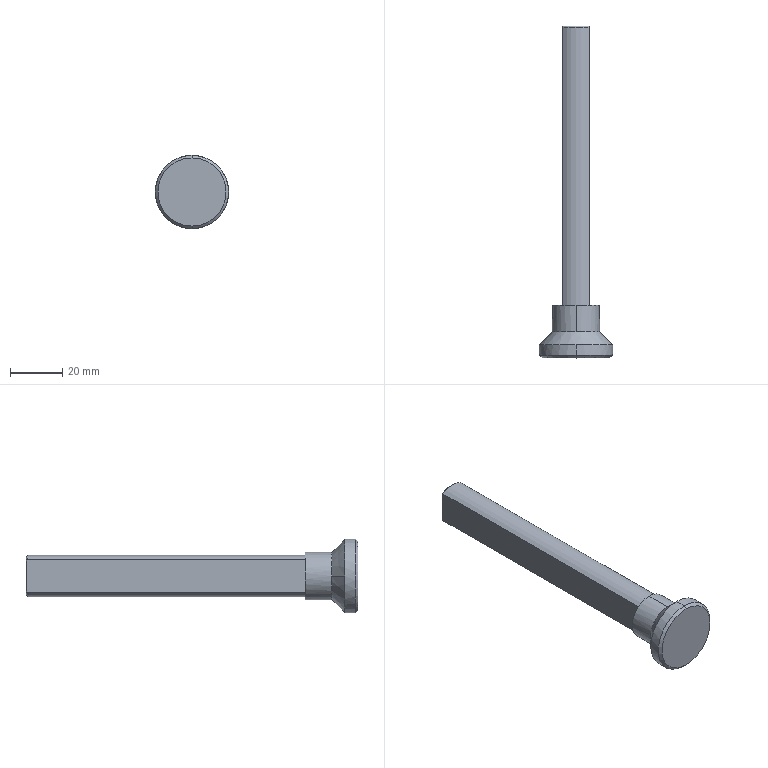Part | STEP file | PN_0017 Snap-ring stop plate | 1 solid | 19 faces | box 28 x 126.5 x 28 mm | volume 23542 mm3 | cylinder 7 | cone 7 | plane 5 | commonest cylinder face diameters 16 x3 18 x2 28 x2
STEP:
#1=CARTESIAN_POINT('',(0.,0.,0.));
#2=DIRECTION('',(0.,0.,1.));
#3=DIRECTION('',(1.,0.,0.));
#4=AXIS2_PLACEMENT_3D('',#1,#2,#3);
#5=CARTESIAN_POINT('',(-5.,106.,-6.245));
#6=VERTEX_POINT('',#5);
#7=CARTESIAN_POINT('',(0.,106.,-8.));
#8=VERTEX_POINT('',#7);
#9=CARTESIAN_POINT('',(0.,106.,0.));
#10=DIRECTION('',(0.,-1.,0.));
#11=DIRECTION('',(0.,0.,-1.));
#12=AXIS2_PLACEMENT_3D('',#9,#10,#11);
#13=CIRCLE('',#12,8.);
#14=CARTESIAN_POINT('',(0.,106.5,0.));
#15=DIRECTION('',(0.,-1.,0.));
#16=DIRECTION('',(0.,0.,-1.));
#17=AXIS2_PLACEMENT_3D('',#14,#15,#16);
#18=CYLINDRICAL_SURFACE('',#17,8.);
#19=CARTESIAN_POINT('',(0.,0.5));
#20=DIRECTION('',(1.,0.));
#21=VECTOR('',#20,1.);
#22=LINE('',#19,#21);
#23=(GEOMETRIC_REPRESENTATION_CONTEXT(2)PARAMETRIC_REPRESENTATION_CONTEXT()REPRESENTATION_CONTEXT('',''));
#24=DEFINITIONAL_REPRESENTATION('',(#22),#23);
#25=PCURVE('',#18,#24);
#26=CARTESIAN_POINT('',(0.,106.,0.));
#27=DIRECTION('',(0.,-1.,0.));
#28=DIRECTION('',(0.,0.,-1.));
#29=AXIS2_PLACEMENT_3D('',#26,#27,#28);
#30=CONICAL_SURFACE('',#29,8.,0.7854);
#31=CARTESIAN_POINT('',(0.,0.));
#32=DIRECTION('',(1.,0.));
#33=VECTOR('',#32,1.);
#34=LINE('',#31,#33);
#35=(GEOMETRIC_REPRESENTATION_CONTEXT(2)PARAMETRIC_REPRESENTATION_CONTEXT()REPRESENTATION_CONTEXT('',''));
#36=DEFINITIONAL_REPRESENTATION('',(#34),#35);
#37=PCURVE('',#30,#36);
#38=SURFACE_CURVE('',#13,(#25,#37),.PCURVE_S1.);
#39=EDGE_CURVE('',#6,#8,#38,.T.);
#40=ORIENTED_EDGE('',*,*,#39,.T.);
#41=CARTESIAN_POINT('',(0.,0.,-8.));
#42=VERTEX_POINT('',#41);
#43=CARTESIAN_POINT('',(0.,106.5,-8.));
#44=DIRECTION('',(0.,-1.,0.));
#45=VECTOR('',#44,1.);
#46=LINE('',#43,#45);
#47=CARTESIAN_POINT('',(6.283,0.));
#48=DIRECTION('',(0.,1.));
#49=VECTOR('',#48,1.);
#50=LINE('',#47,#49);
#51=(GEOMETRIC_REPRESENTATION_CONTEXT(2)PARAMETRIC_REPRESENTATION_CONTEXT()REPRESENTATION_CONTEXT('',''));
#52=DEFINITIONAL_REPRESENTATION('',(#50),#51);
#53=PCURVE('',#18,#52);
#54=CARTESIAN_POINT('',(0.,106.5,0.));
#55=DIRECTION('',(0.,-1.,0.));
#56=DIRECTION('',(0.,0.,-1.));
#57=AXIS2_PLACEMENT_3D('',#54,#55,#56);
#58=CYLINDRICAL_SURFACE('',#57,8.);
#59=CARTESIAN_POINT('',(0.,0.));
#60=DIRECTION('',(0.,1.));
#61=VECTOR('',#60,1.);
#62=LINE('',#59,#61);
#63=(GEOMETRIC_REPRESENTATION_CONTEXT(2)PARAMETRIC_REPRESENTATION_CONTEXT()REPRESENTATION_CONTEXT('',''));
#64=DEFINITIONAL_REPRESENTATION('',(#62),#63);
#65=PCURVE('',#58,#64);
#66=SURFACE_CURVE('',#46,(#53,#65),.PCURVE_S1.);
#67=EDGE_CURVE('',#8,#42,#66,.T.);
#68=ORIENTED_EDGE('',*,*,#67,.T.);
#69=CARTESIAN_POINT('',(-5.,0.,-6.245));
#70=VERTEX_POINT('',#69);
#71=CARTESIAN_POINT('',(0.,0.,0.));
#72=DIRECTION('',(0.,1.,0.));
#73=DIRECTION('',(0.,0.,-1.));
#74=AXIS2_PLACEMENT_3D('',#71,#72,#73);
#75=CIRCLE('',#74,8.);
#76=CARTESIAN_POINT('',(6.283,106.5));
#77=DIRECTION('',(-1.,0.));
#78=VECTOR('',#77,1.);
#79=LINE('',#76,#78);
#80=(GEOMETRIC_REPRESENTATION_CONTEXT(2)PARAMETRIC_REPRESENTATION_CONTEXT()REPRESENTATION_CONTEXT('',''));
#81=DEFINITIONAL_REPRESENTATION('',(#79),#80);
#82=PCURVE('',#18,#81);
#83=CARTESIAN_POINT('',(0.,0.,0.));
#84=DIRECTION('',(0.,-1.,0.));
#85=DIRECTION('',(0.,0.,-1.));
#86=AXIS2_PLACEMENT_3D('',#83,#84,#85);
#87=PLANE('',#86);
#88=CARTESIAN_POINT('',(8.,0.));
#89=CARTESIAN_POINT('',(8.,-13.856));
#90=CARTESIAN_POINT('',(-4.,-6.928));
#91=CARTESIAN_POINT('',(-16.,0.));
#92=CARTESIAN_POINT('',(-4.,6.928));
#93=CARTESIAN_POINT('',(8.,13.856));
#94=CARTESIAN_POINT('',(8.,0.));
#95=(BOUNDED_CURVE()B_SPLINE_CURVE(2,(#88,#89,#90,#91,#92,#93,#94),.UNSPECIFIED.,.T.,.F.)B_SPLINE_CURVE_WITH_KNOTS((1,2,2,2,2,1),(-2.094,0.,2.094,4.189,6.283,8.378),.UNSPECIFIED.)CURVE()GEOMETRIC_REPRESENTATION_ITEM()RATIONAL_B_SPLINE_CURVE((1.,0.5,1.,0.5,1.,0.5,1.))REPRESENTATION_ITEM(''));
#96=(GEOMETRIC_REPRESENTATION_CONTEXT(2)PARAMETRIC_REPRESENTATION_CONTEXT()REPRESENTATION_CONTEXT('',''));
#97=DEFINITIONAL_REPRESENTATION('',(#95),#96);
#98=PCURVE('',#87,#97);
#99=SURFACE_CURVE('',#75,(#82,#98),.PCURVE_S1.);
#100=EDGE_CURVE('',#42,#70,#99,.T.);
#101=ORIENTED_EDGE('',*,*,#100,.T.);
#102=CARTESIAN_POINT('',(-5.,-39.994,-6.245));
#103=DIRECTION('',(0.,-1.,0.));
#104=VECTOR('',#103,1.);
#105=LINE('',#102,#104);
#106=CARTESIAN_POINT('',(5.608,146.494));
#107=DIRECTION('',(0.,1.));
#108=VECTOR('',#107,1.);
#109=LINE('',#106,#108);
#110=(GEOMETRIC_REPRESENTATION_CONTEXT(2)PARAMETRIC_REPRESENTATION_CONTEXT()REPRESENTATION_CONTEXT('',''));
#111=DEFINITIONAL_REPRESENTATION('',(#109),#110);
#112=PCURVE('',#18,#111);
#113=CARTESIAN_POINT('',(-5.,-39.994,-10.));
#114=DIRECTION('',(-1.,0.,0.));
#115=DIRECTION('',(0.,0.,1.));
#116=AXIS2_PLACEMENT_3D('',#113,#114,#115);
#117=PLANE('',#116);
#118=CARTESIAN_POINT('',(3.755,0.));
#119=DIRECTION('',(0.,-1.));
#120=VECTOR('',#119,1.);
#121=LINE('',#118,#120);
#122=(GEOMETRIC_REPRESENTATION_CONTEXT(2)PARAMETRIC_REPRESENTATION_CONTEXT()REPRESENTATION_CONTEXT('',''));
#123=DEFINITIONAL_REPRESENTATION('',(#121),#122);
#124=PCURVE('',#117,#123);
#125=SURFACE_CURVE('',#105,(#112,#124),.PCURVE_S1.);
#126=EDGE_CURVE('',#6,#70,#125,.T.);
#127=ORIENTED_EDGE('',*,*,#126,.F.);
#128=EDGE_LOOP('',(#40,#68,#101,#127));
#129=FACE_BOUND('',#128,.T.);
#130=ADVANCED_FACE('',(#129),#18,.T.);
#131=CARTESIAN_POINT('',(0.,106.5,-7.5));
#132=VERTEX_POINT('',#131);
#133=CARTESIAN_POINT('',(-5.,106.5,-5.59));
#134=VERTEX_POINT('',#133);
#135=CARTESIAN_POINT('',(0.,106.5,0.));
#136=DIRECTION('',(0.,1.,0.));
#137=DIRECTION('',(0.,0.,-1.));
#138=AXIS2_PLACEMENT_3D('',#135,#136,#137);
#139=CIRCLE('',#138,7.5);
#140=CARTESIAN_POINT('',(6.283,-0.5));
#141=DIRECTION('',(-1.,0.));
#142=VECTOR('',#141,1.);
#143=LINE('',#140,#142);
#144=(GEOMETRIC_REPRESENTATION_CONTEXT(2)PARAMETRIC_REPRESENTATION_CONTEXT()REPRESENTATION_CONTEXT('',''));
#145=DEFINITIONAL_REPRESENTATION('',(#143),#144);
#146=PCURVE('',#30,#145);
#147=CARTESIAN_POINT('',(0.,106.5,0.));
#148=DIRECTION('',(0.,1.,0.));
#149=DIRECTION('',(0.,0.,1.));
#150=AXIS2_PLACEMENT_3D('',#147,#148,#149);
#151=PLANE('',#150);
#152=CARTESIAN_POINT('',(0.,0.));
#153=DIRECTION('',(-1.,0.));
#154=AXIS2_PLACEMENT_2D('',#152,#153);
#155=CIRCLE('',#154,7.5);
#156=(GEOMETRIC_REPRESENTATION_CONTEXT(2)PARAMETRIC_REPRESENTATION_CONTEXT()REPRESENTATION_CONTEXT('',''));
#157=DEFINITIONAL_REPRESENTATION('',(#155),#156);
#158=PCURVE('',#151,#157);
#159=SURFACE_CURVE('',#139,(#146,#158),.PCURVE_S1.);
#160=EDGE_CURVE('',#132,#134,#159,.T.);
#161=ORIENTED_EDGE('',*,*,#160,.F.);
#162=CARTESIAN_POINT('',(0.,106.,-8.));
#163=DIRECTION('',(0.,-0.7071,-0.7071));
#164=VECTOR('',#163,1.);
#165=LINE('',#162,#164);
#166=CARTESIAN_POINT('',(6.283,0.));
#167=DIRECTION('',(0.,1.));
#168=VECTOR('',#167,1.);
#169=LINE('',#166,#168);
#170=(GEOMETRIC_REPRESENTATION_CONTEXT(2)PARAMETRIC_REPRESENTATION_CONTEXT()REPRESENTATION_CONTEXT('',''));
#171=DEFINITIONAL_REPRESENTATION('',(#169),#170);
#172=PCURVE('',#30,#171);
#173=CARTESIAN_POINT('',(0.,106.,0.));
#174=DIRECTION('',(0.,-1.,0.));
#175=DIRECTION('',(0.,0.,-1.));
#176=AXIS2_PLACEMENT_3D('',#173,#174,#175);
#177=CONICAL_SURFACE('',#176,8.,0.7854);
#178=CARTESIAN_POINT('',(0.,0.));
#179=DIRECTION('',(0.,1.));
#180=VECTOR('',#179,1.);
#181=LINE('',#178,#180);
#182=(GEOMETRIC_REPRESENTATION_CONTEXT(2)PARAMETRIC_REPRESENTATION_CONTEXT()REPRESENTATION_CONTEXT('',''));
#183=DEFINITIONAL_REPRESENTATION('',(#181),#182);
#184=PCURVE('',#177,#183);
#185=SURFACE_CURVE('',#165,(#172,#184),.PCURVE_S1.);
#186=EDGE_CURVE('',#132,#8,#185,.T.);
#187=ORIENTED_EDGE('',*,*,#186,.T.);
#188=ORIENTED_EDGE('',*,*,#39,.F.);
#189=CARTESIAN_POINT('',(-5.,106.,-6.245));
#190=CARTESIAN_POINT('',(-5.,106.169,-6.029));
#191=CARTESIAN_POINT('',(-5.,106.336,-5.81));
#192=CARTESIAN_POINT('',(-5.,106.5,-5.59));
#193=B_SPLINE_CURVE_WITH_KNOTS('',3,(#189,#190,#191,#192),.UNSPECIFIED.,.F.,.F.,(4,4),(0.,0.0008239),.PIECEWISE_BEZIER_KNOTS.);
#194=CARTESIAN_POINT('',(5.608,0.));
#195=CARTESIAN_POINT('',(5.607,-0.007681));
#196=CARTESIAN_POINT('',(5.606,-0.02304));
#197=CARTESIAN_POINT('',(5.603,-0.04604));
#198=CARTESIAN_POINT('',(5.601,-0.06902));
#199=CARTESIAN_POINT('',(5.599,-0.09197));
#200=CARTESIAN_POINT('',(5.596,-0.1149));
#201=CARTESIAN_POINT('',(5.594,-0.1378));
#202=CARTESIAN_POINT('',(5.592,-0.1607));
#203=CARTESIAN_POINT('',(5.589,-0.1835));
#204=CARTESIAN_POINT('',(5.587,-0.2063));
#205=CARTESIAN_POINT('',(5.584,-0.2291));
#206=CARTESIAN_POINT('',(5.582,-0.2518));
#207=CARTESIAN_POINT('',(5.579,-0.2745));
#208=CARTESIAN_POINT('',(5.577,-0.2972));
#209=CARTESIAN_POINT('',(5.574,-0.3199));
#210=CARTESIAN_POINT('',(5.572,-0.3425));
#211=CARTESIAN_POINT('',(5.569,-0.3651));
#212=CARTESIAN_POINT('',(5.567,-0.3877));
#213=CARTESIAN_POINT('',(5.564,-0.4102));
#214=CARTESIAN_POINT('',(5.561,-0.4327));
#215=CARTESIAN_POINT('',(5.559,-0.4552));
#216=CARTESIAN_POINT('',(5.556,-0.4776));
#217=CARTESIAN_POINT('',(5.554,-0.4925));
#218=CARTESIAN_POINT('',(5.553,-0.5));
#219=B_SPLINE_CURVE_WITH_KNOTS('',3,(#194,#195,#196,#197,#198,#199,#200,#201,#202,#203,#204,#205,#206,#207,#208,#209,#210,#211,#212,#213,#214,#215,#216,#217,#218),.UNSPECIFIED.,.F.,.F.,(4,1,1,1,1,1,1,1,1,1,1,1,1,1,1,1,1,1,1,1,1,1,4),(0.,0.00003745,0.0000749,0.0001123,0.0001498,0.0001872,0.0002247,0.0002621,0.0002996,0.000337,0.0003745,0.0004119,0.0004494,0.0004868,0.0005243,0.0005617,0.0005992,0.0006366,0.0006741,0.0007115,0.000749,0.0007864,0.0008239),.QUASI_UNIFORM_KNOTS.);
#220=(GEOMETRIC_REPRESENTATION_CONTEXT(2)PARAMETRIC_REPRESENTATION_CONTEXT()REPRESENTATION_CONTEXT('',''));
#221=DEFINITIONAL_REPRESENTATION('',(#219),#220);
#222=PCURVE('',#30,#221);
#223=CARTESIAN_POINT('',(3.755,145.994));
#224=CARTESIAN_POINT('',(3.971,146.163));
#225=CARTESIAN_POINT('',(4.19,146.33));
#226=CARTESIAN_POINT('',(4.41,146.494));
#227=B_SPLINE_CURVE_WITH_KNOTS('',3,(#223,#224,#225,#226),.UNSPECIFIED.,.F.,.F.,(4,4),(0.,0.0008239),.PIECEWISE_BEZIER_KNOTS.);
#228=(GEOMETRIC_REPRESENTATION_CONTEXT(2)PARAMETRIC_REPRESENTATION_CONTEXT()REPRESENTATION_CONTEXT('',''));
#229=DEFINITIONAL_REPRESENTATION('',(#227),#228);
#230=PCURVE('',#117,#229);
#231=SURFACE_CURVE('',#193,(#222,#230),.PCURVE_S1.);
#232=EDGE_CURVE('',#6,#134,#231,.T.);
#233=ORIENTED_EDGE('',*,*,#232,.T.);
#234=EDGE_LOOP('',(#161,#187,#188,#233));
#235=FACE_BOUND('',#234,.T.);
#236=ADVANCED_FACE('',(#235),#30,.T.);
#237=CARTESIAN_POINT('',(9.,-10.,0.));
#238=VERTEX_POINT('',#237);
#239=CARTESIAN_POINT('',(0.,-10.,-9.));
#240=VERTEX_POINT('',#239);
#241=CARTESIAN_POINT('',(0.,-10.,0.));
#242=DIRECTION('',(0.,1.,0.));
#243=DIRECTION('',(0.,0.,1.));
#244=AXIS2_PLACEMENT_3D('',#241,#242,#243);
#245=CIRCLE('',#244,9.);
#246=CARTESIAN_POINT('',(0.,-15.,0.));
#247=DIRECTION('',(0.,1.,0.));
#248=DIRECTION('',(0.,0.,1.));
#249=AXIS2_PLACEMENT_3D('',#246,#247,#248);
#250=CYLINDRICAL_SURFACE('',#249,9.);
#251=CARTESIAN_POINT('',(0.,5.));
#252=DIRECTION('',(1.,0.));
#253=VECTOR('',#252,1.);
#254=LINE('',#251,#253);
#255=(GEOMETRIC_REPRESENTATION_CONTEXT(2)PARAMETRIC_REPRESENTATION_CONTEXT()REPRESENTATION_CONTEXT('',''));
#256=DEFINITIONAL_REPRESENTATION('',(#254),#255);
#257=PCURVE('',#250,#256);
#258=CARTESIAN_POINT('',(0.,-15.,0.));
#259=DIRECTION('',(0.,-1.,0.));
#260=DIRECTION('',(1.,0.,0.));
#261=AXIS2_PLACEMENT_3D('',#258,#259,#260);
#262=CONICAL_SURFACE('',#261,14.,0.7854);
#263=CARTESIAN_POINT('',(7.854,-5.));
#264=DIRECTION('',(-1.,0.));
#265=VECTOR('',#264,1.);
#266=LINE('',#263,#265);
#267=(GEOMETRIC_REPRESENTATION_CONTEXT(2)PARAMETRIC_REPRESENTATION_CONTEXT()REPRESENTATION_CONTEXT('',''));
#268=DEFINITIONAL_REPRESENTATION('',(#266),#267);
#269=PCURVE('',#262,#268);
#270=SURFACE_CURVE('',#245,(#257,#269),.PCURVE_S1.);
#271=EDGE_CURVE('',#238,#240,#270,.T.);
#272=ORIENTED_EDGE('',*,*,#271,.T.);
#273=CARTESIAN_POINT('',(0.,0.,-9.));
#274=VERTEX_POINT('',#273);
#275=CARTESIAN_POINT('',(0.,-15.,-9.));
#276=DIRECTION('',(0.,1.,0.));
#277=VECTOR('',#276,1.);
#278=LINE('',#275,#277);
#279=CARTESIAN_POINT('',(3.142,0.));
#280=DIRECTION('',(0.,1.));
#281=VECTOR('',#280,1.);
#282=LINE('',#279,#281);
#283=(GEOMETRIC_REPRESENTATION_CONTEXT(2)PARAMETRIC_REPRESENTATION_CONTEXT()REPRESENTATION_CONTEXT('',''));
#284=DEFINITIONAL_REPRESENTATION('',(#282),#283);
#285=PCURVE('',#250,#284);
#286=CARTESIAN_POINT('',(0.,-15.,0.));
#287=DIRECTION('',(0.,1.,0.));
#288=DIRECTION('',(0.,0.,1.));
#289=AXIS2_PLACEMENT_3D('',#286,#287,#288);
#290=CYLINDRICAL_SURFACE('',#289,9.);
#291=CARTESIAN_POINT('',(3.142,0.));
#292=DIRECTION('',(0.,1.));
#293=VECTOR('',#292,1.);
#294=LINE('',#291,#293);
#295=(GEOMETRIC_REPRESENTATION_CONTEXT(2)PARAMETRIC_REPRESENTATION_CONTEXT()REPRESENTATION_CONTEXT('',''));
#296=DEFINITIONAL_REPRESENTATION('',(#294),#295);
#297=PCURVE('',#290,#296);
#298=SURFACE_CURVE('',#278,(#285,#297),.PCURVE_S1.);
#299=EDGE_CURVE('',#240,#274,#298,.T.);
#300=ORIENTED_EDGE('',*,*,#299,.T.);
#301=CARTESIAN_POINT('',(0.,0.,9.));
#302=VERTEX_POINT('',#301);
#303=CARTESIAN_POINT('',(0.,0.,0.));
#304=DIRECTION('',(0.,-1.,0.));
#305=DIRECTION('',(0.,0.,1.));
#306=AXIS2_PLACEMENT_3D('',#303,#304,#305);
#307=CIRCLE('',#306,9.);
#308=CARTESIAN_POINT('',(6.283,15.));
#309=DIRECTION('',(-1.,0.));
#310=VECTOR('',#309,1.);
#311=LINE('',#308,#310);
#312=(GEOMETRIC_REPRESENTATION_CONTEXT(2)PARAMETRIC_REPRESENTATION_CONTEXT()REPRESENTATION_CONTEXT('',''));
#313=DEFINITIONAL_REPRESENTATION('',(#311),#312);
#314=PCURVE('',#250,#313);
#315=CARTESIAN_POINT('',(0.,0.));
#316=DIRECTION('',(-1.,0.));
#317=AXIS2_PLACEMENT_2D('',#315,#316);
#318=CIRCLE('',#317,9.);
#319=(GEOMETRIC_REPRESENTATION_CONTEXT(2)PARAMETRIC_REPRESENTATION_CONTEXT()REPRESENTATION_CONTEXT('',''));
#320=DEFINITIONAL_REPRESENTATION('',(#318),#319);
#321=PCURVE('',#87,#320);
#322=SURFACE_CURVE('',#307,(#314,#321),.PCURVE_S1.);
#323=EDGE_CURVE('',#274,#302,#322,.T.);
#324=ORIENTED_EDGE('',*,*,#323,.T.);
#325=CARTESIAN_POINT('',(0.,-10.,9.));
#326=VERTEX_POINT('',#325);
#327=CARTESIAN_POINT('',(0.,-15.,9.));
#328=DIRECTION('',(0.,1.,0.));
#329=VECTOR('',#328,1.);
#330=LINE('',#327,#329);
#331=CARTESIAN_POINT('',(0.,0.));
#332=DIRECTION('',(0.,1.));
#333=VECTOR('',#332,1.);
#334=LINE('',#331,#333);
#335=(GEOMETRIC_REPRESENTATION_CONTEXT(2)PARAMETRIC_REPRESENTATION_CONTEXT()REPRESENTATION_CONTEXT('',''));
#336=DEFINITIONAL_REPRESENTATION('',(#334),#335);
#337=PCURVE('',#250,#336);
#338=CARTESIAN_POINT('',(6.283,0.));
#339=DIRECTION('',(0.,1.));
#340=VECTOR('',#339,1.);
#341=LINE('',#338,#340);
#342=(GEOMETRIC_REPRESENTATION_CONTEXT(2)PARAMETRIC_REPRESENTATION_CONTEXT()REPRESENTATION_CONTEXT('',''));
#343=DEFINITIONAL_REPRESENTATION('',(#341),#342);
#344=PCURVE('',#290,#343);
#345=SURFACE_CURVE('',#330,(#337,#344),.PCURVE_S1.);
#346=EDGE_CURVE('',#326,#302,#345,.T.);
#347=ORIENTED_EDGE('',*,*,#346,.F.);
#348=CARTESIAN_POINT('',(0.,-10.,0.));
#349=DIRECTION('',(0.,1.,0.));
#350=DIRECTION('',(0.,0.,1.));
#351=AXIS2_PLACEMENT_3D('',#348,#349,#350);
#352=CIRCLE('',#351,9.);
#353=CARTESIAN_POINT('',(0.,5.));
#354=DIRECTION('',(1.,0.));
#355=VECTOR('',#354,1.);
#356=LINE('',#353,#355);
#357=(GEOMETRIC_REPRESENTATION_CONTEXT(2)PARAMETRIC_REPRESENTATION_CONTEXT()REPRESENTATION_CONTEXT('',''));
#358=DEFINITIONAL_REPRESENTATION('',(#356),#357);
#359=PCURVE('',#250,#358);
#360=CARTESIAN_POINT('',(0.,-15.,0.));
#361=DIRECTION('',(0.,-1.,0.));
#362=DIRECTION('',(1.,0.,0.));
#363=AXIS2_PLACEMENT_3D('',#360,#361,#362);
#364=CONICAL_SURFACE('',#363,14.,0.7854);
#365=CARTESIAN_POINT('',(1.571,-5.));
#366=DIRECTION('',(-1.,0.));
#367=VECTOR('',#366,1.);
#368=LINE('',#365,#367);
#369=(GEOMETRIC_REPRESENTATION_CONTEXT(2)PARAMETRIC_REPRESENTATION_CONTEXT()REPRESENTATION_CONTEXT('',''));
#370=DEFINITIONAL_REPRESENTATION('',(#368),#369);
#371=PCURVE('',#364,#370);
#372=SURFACE_CURVE('',#352,(#359,#371),.PCURVE_S1.);
#373=EDGE_CURVE('',#326,#238,#372,.T.);
#374=ORIENTED_EDGE('',*,*,#373,.T.);
#375=EDGE_LOOP('',(#272,#300,#324,#347,#374));
#376=FACE_BOUND('',#375,.T.);
#377=ADVANCED_FACE('',(#376),#250,.T.);
#378=CARTESIAN_POINT('',(-9.,-10.,0.));
#379=VERTEX_POINT('',#378);
#380=CARTESIAN_POINT('',(0.,-10.,0.));
#381=DIRECTION('',(0.,1.,0.));
#382=DIRECTION('',(0.,0.,1.));
#383=AXIS2_PLACEMENT_3D('',#380,#381,#382);
#384=CIRCLE('',#383,9.);
#385=CARTESIAN_POINT('',(7.854,-5.));
#386=DIRECTION('',(-1.,0.));
#387=VECTOR('',#386,1.);
#388=LINE('',#385,#387);
#389=(GEOMETRIC_REPRESENTATION_CONTEXT(2)PARAMETRIC_REPRESENTATION_CONTEXT()REPRESENTATION_CONTEXT('',''));
#390=DEFINITIONAL_REPRESENTATION('',(#388),#389);
#391=PCURVE('',#364,#390);
#392=CARTESIAN_POINT('',(0.,5.));
#393=DIRECTION('',(1.,0.));
#394=VECTOR('',#393,1.);
#395=LINE('',#392,#394);
#396=(GEOMETRIC_REPRESENTATION_CONTEXT(2)PARAMETRIC_REPRESENTATION_CONTEXT()REPRESENTATION_CONTEXT('',''));
#397=DEFINITIONAL_REPRESENTATION('',(#395),#396);
#398=PCURVE('',#290,#397);
#399=SURFACE_CURVE('',#384,(#391,#398),.PCURVE_S1.);
#400=EDGE_CURVE('',#379,#326,#399,.T.);
#401=ORIENTED_EDGE('',*,*,#400,.F.);
#402=CARTESIAN_POINT('',(-14.,-15.,0.));
#403=VERTEX_POINT('',#402);
#404=CARTESIAN_POINT('',(-14.,-15.,0.));
#405=DIRECTION('',(-0.7071,-0.7071,0.));
#406=VECTOR('',#405,1.);
#407=LINE('',#404,#406);
#408=CARTESIAN_POINT('',(3.142,0.));
#409=DIRECTION('',(0.,1.));
#410=VECTOR('',#409,1.);
#411=LINE('',#408,#410);
#412=(GEOMETRIC_REPRESENTATION_CONTEXT(2)PARAMETRIC_REPRESENTATION_CONTEXT()REPRESENTATION_CONTEXT('',''));
#413=DEFINITIONAL_REPRESENTATION('',(#411),#412);
#414=PCURVE('',#364,#413);
#415=CARTESIAN_POINT('',(3.142,0.));
#416=DIRECTION('',(0.,1.));
#417=VECTOR('',#416,1.);
#418=LINE('',#415,#417);
#419=(GEOMETRIC_REPRESENTATION_CONTEXT(2)PARAMETRIC_REPRESENTATION_CONTEXT()REPRESENTATION_CONTEXT('',''));
#420=DEFINITIONAL_REPRESENTATION('',(#418),#419);
#421=PCURVE('',#262,#420);
#422=SURFACE_CURVE('',#407,(#414,#421),.PCURVE_S1.);
#423=EDGE_CURVE('',#379,#403,#422,.T.);
#424=ORIENTED_EDGE('',*,*,#423,.T.);
#425=CARTESIAN_POINT('',(0.,-15.,14.));
#426=VERTEX_POINT('',#425);
#427=CARTESIAN_POINT('',(0.,-15.,0.));
#428=DIRECTION('',(0.,1.,0.));
#429=DIRECTION('',(0.,0.,-1.));
#430=AXIS2_PLACEMENT_3D('',#427,#428,#429);
#431=CIRCLE('',#430,14.);
#432=CARTESIAN_POINT('',(4.712,0.));
#433=DIRECTION('',(-1.,0.));
#434=VECTOR('',#433,1.);
#435=LINE('',#432,#434);
#436=(GEOMETRIC_REPRESENTATION_CONTEXT(2)PARAMETRIC_REPRESENTATION_CONTEXT()REPRESENTATION_CONTEXT('',''));
#437=DEFINITIONAL_REPRESENTATION('',(#435),#436);
#438=PCURVE('',#364,#437);
#439=CARTESIAN_POINT('',(0.,-20.,0.));
#440=DIRECTION('',(0.,1.,0.));
#441=DIRECTION('',(0.,0.,1.));
#442=AXIS2_PLACEMENT_3D('',#439,#440,#441);
#443=CYLINDRICAL_SURFACE('',#442,14.);
#444=CARTESIAN_POINT('',(3.142,5.));
#445=DIRECTION('',(1.,0.));
#446=VECTOR('',#445,1.);
#447=LINE('',#444,#446);
#448=(GEOMETRIC_REPRESENTATION_CONTEXT(2)PARAMETRIC_REPRESENTATION_CONTEXT()REPRESENTATION_CONTEXT('',''));
#449=DEFINITIONAL_REPRESENTATION('',(#447),#448);
#450=PCURVE('',#443,#449);
#451=SURFACE_CURVE('',#431,(#438,#450),.PCURVE_S1.);
#452=EDGE_CURVE('',#403,#426,#451,.T.);
#453=ORIENTED_EDGE('',*,*,#452,.T.);
#454=CARTESIAN_POINT('',(14.,-15.,0.));
#455=VERTEX_POINT('',#454);
#456=CARTESIAN_POINT('',(0.,-15.,0.));
#457=DIRECTION('',(0.,1.,0.));
#458=DIRECTION('',(0.,0.,-1.));
#459=AXIS2_PLACEMENT_3D('',#456,#457,#458);
#460=CIRCLE('',#459,14.);
#461=CARTESIAN_POINT('',(4.712,0.));
#462=DIRECTION('',(-1.,0.));
#463=VECTOR('',#462,1.);
#464=LINE('',#461,#463);
#465=(GEOMETRIC_REPRESENTATION_CONTEXT(2)PARAMETRIC_REPRESENTATION_CONTEXT()REPRESENTATION_CONTEXT('',''));
#466=DEFINITIONAL_REPRESENTATION('',(#464),#465);
#467=PCURVE('',#364,#466);
#468=CARTESIAN_POINT('',(0.,-20.,0.));
#469=DIRECTION('',(0.,1.,0.));
#470=DIRECTION('',(0.,0.,1.));
#471=AXIS2_PLACEMENT_3D('',#468,#469,#470);
#472=CYLINDRICAL_SURFACE('',#471,14.);
#473=CARTESIAN_POINT('',(-3.142,5.));
#474=DIRECTION('',(1.,0.));
#475=VECTOR('',#474,1.);
#476=LINE('',#473,#475);
#477=(GEOMETRIC_REPRESENTATION_CONTEXT(2)PARAMETRIC_REPRESENTATION_CONTEXT()REPRESENTATION_CONTEXT('',''));
#478=DEFINITIONAL_REPRESENTATION('',(#476),#477);
#479=PCURVE('',#472,#478);
#480=SURFACE_CURVE('',#460,(#467,#479),.PCURVE_S1.);
#481=EDGE_CURVE('',#426,#455,#480,.T.);
#482=ORIENTED_EDGE('',*,*,#481,.T.);
#483=CARTESIAN_POINT('',(14.,-15.,0.));
#484=DIRECTION('',(0.7071,-0.7071,0.));
#485=VECTOR('',#484,1.);
#486=LINE('',#483,#485);
#487=CARTESIAN_POINT('',(0.,0.));
#488=DIRECTION('',(0.,1.));
#489=VECTOR('',#488,1.);
#490=LINE('',#487,#489);
#491=(GEOMETRIC_REPRESENTATION_CONTEXT(2)PARAMETRIC_REPRESENTATION_CONTEXT()REPRESENTATION_CONTEXT('',''));
#492=DEFINITIONAL_REPRESENTATION('',(#490),#491);
#493=PCURVE('',#364,#492);
#494=CARTESIAN_POINT('',(6.283,0.));
#495=DIRECTION('',(0.,1.));
#496=VECTOR('',#495,1.);
#497=LINE('',#494,#496);
#498=(GEOMETRIC_REPRESENTATION_CONTEXT(2)PARAMETRIC_REPRESENTATION_CONTEXT()REPRESENTATION_CONTEXT('',''));
#499=DEFINITIONAL_REPRESENTATION('',(#497),#498);
#500=PCURVE('',#262,#499);
#501=SURFACE_CURVE('',#486,(#493,#500),.PCURVE_S1.);
#502=EDGE_CURVE('',#238,#455,#501,.T.);
#503=ORIENTED_EDGE('',*,*,#502,.F.);
#504=ORIENTED_EDGE('',*,*,#373,.F.);
#505=EDGE_LOOP('',(#401,#424,#453,#482,#503,#504));
#506=FACE_BOUND('',#505,.T.);
#507=ADVANCED_FACE('',(#506),#364,.T.);
#508=CARTESIAN_POINT('',(0.,-19.,14.));
#509=VERTEX_POINT('',#508);
#510=CARTESIAN_POINT('',(0.,-19.,-14.));
#511=VERTEX_POINT('',#510);
#512=CARTESIAN_POINT('',(0.,-19.,0.));
#513=DIRECTION('',(0.,1.,0.));
#514=DIRECTION('',(0.,0.,1.));
#515=AXIS2_PLACEMENT_3D('',#512,#513,#514);
#516=CIRCLE('',#515,14.);
#517=CARTESIAN_POINT('',(0.,1.));
#518=DIRECTION('',(1.,0.));
#519=VECTOR('',#518,1.);
#520=LINE('',#517,#519);
#521=(GEOMETRIC_REPRESENTATION_CONTEXT(2)PARAMETRIC_REPRESENTATION_CONTEXT()REPRESENTATION_CONTEXT('',''));
#522=DEFINITIONAL_REPRESENTATION('',(#520),#521);
#523=PCURVE('',#472,#522);
#524=CARTESIAN_POINT('',(0.,-19.,0.));
#525=DIRECTION('',(0.,1.,0.));
#526=DIRECTION('',(0.,0.,1.));
#527=AXIS2_PLACEMENT_3D('',#524,#525,#526);
#528=CONICAL_SURFACE('',#527,14.,0.7854);
#529=CARTESIAN_POINT('',(0.,0.));
#530=DIRECTION('',(1.,0.));
#531=VECTOR('',#530,1.);
#532=LINE('',#529,#531);
#533=(GEOMETRIC_REPRESENTATION_CONTEXT(2)PARAMETRIC_REPRESENTATION_CONTEXT()REPRESENTATION_CONTEXT('',''));
#534=DEFINITIONAL_REPRESENTATION('',(#532),#533);
#535=PCURVE('',#528,#534);
#536=SURFACE_CURVE('',#516,(#523,#535),.PCURVE_S1.);
#537=EDGE_CURVE('',#509,#511,#536,.T.);
#538=ORIENTED_EDGE('',*,*,#537,.T.);
#539=CARTESIAN_POINT('',(0.,-15.,-14.));
#540=VERTEX_POINT('',#539);
#541=CARTESIAN_POINT('',(0.,-20.,-14.));
#542=DIRECTION('',(0.,1.,0.));
#543=VECTOR('',#542,1.);
#544=LINE('',#541,#543);
#545=CARTESIAN_POINT('',(3.142,0.));
#546=DIRECTION('',(0.,1.));
#547=VECTOR('',#546,1.);
#548=LINE('',#545,#547);
#549=(GEOMETRIC_REPRESENTATION_CONTEXT(2)PARAMETRIC_REPRESENTATION_CONTEXT()REPRESENTATION_CONTEXT('',''));
#550=DEFINITIONAL_REPRESENTATION('',(#548),#549);
#551=PCURVE('',#472,#550);
#552=CARTESIAN_POINT('',(3.142,0.));
#553=DIRECTION('',(0.,1.));
#554=VECTOR('',#553,1.);
#555=LINE('',#552,#554);
#556=(GEOMETRIC_REPRESENTATION_CONTEXT(2)PARAMETRIC_REPRESENTATION_CONTEXT()REPRESENTATION_CONTEXT('',''));
#557=DEFINITIONAL_REPRESENTATION('',(#555),#556);
#558=PCURVE('',#443,#557);
#559=SURFACE_CURVE('',#544,(#551,#558),.PCURVE_S1.);
#560=EDGE_CURVE('',#511,#540,#559,.T.);
#561=ORIENTED_EDGE('',*,*,#560,.T.);
#562=CARTESIAN_POINT('',(0.,-15.,0.));
#563=DIRECTION('',(0.,1.,0.));
#564=DIRECTION('',(0.,0.,-1.));
#565=AXIS2_PLACEMENT_3D('',#562,#563,#564);
#566=CIRCLE('',#565,14.);
#567=CARTESIAN_POINT('',(-3.142,5.));
#568=DIRECTION('',(1.,0.));
#569=VECTOR('',#568,1.);
#570=LINE('',#567,#569);
#571=(GEOMETRIC_REPRESENTATION_CONTEXT(2)PARAMETRIC_REPRESENTATION_CONTEXT()REPRESENTATION_CONTEXT('',''));
#572=DEFINITIONAL_REPRESENTATION('',(#570),#571);
#573=PCURVE('',#472,#572);
#574=CARTESIAN_POINT('',(10.996,0.));
#575=DIRECTION('',(-1.,0.));
#576=VECTOR('',#575,1.);
#577=LINE('',#574,#576);
#578=(GEOMETRIC_REPRESENTATION_CONTEXT(2)PARAMETRIC_REPRESENTATION_CONTEXT()REPRESENTATION_CONTEXT('',''));
#579=DEFINITIONAL_REPRESENTATION('',(#577),#578);
#580=PCURVE('',#262,#579);
#581=SURFACE_CURVE('',#566,(#573,#580),.PCURVE_S1.);
#582=EDGE_CURVE('',#455,#540,#581,.T.);
#583=ORIENTED_EDGE('',*,*,#582,.F.);
#584=ORIENTED_EDGE('',*,*,#481,.F.);
#585=CARTESIAN_POINT('',(0.,-20.,14.));
#586=DIRECTION('',(0.,1.,0.));
#587=VECTOR('',#586,1.);
#588=LINE('',#585,#587);
#589=CARTESIAN_POINT('',(0.,0.));
#590=DIRECTION('',(0.,1.));
#591=VECTOR('',#590,1.);
#592=LINE('',#589,#591);
#593=(GEOMETRIC_REPRESENTATION_CONTEXT(2)PARAMETRIC_REPRESENTATION_CONTEXT()REPRESENTATION_CONTEXT('',''));
#594=DEFINITIONAL_REPRESENTATION('',(#592),#593);
#595=PCURVE('',#472,#594);
#596=CARTESIAN_POINT('',(6.283,0.));
#597=DIRECTION('',(0.,1.));
#598=VECTOR('',#597,1.);
#599=LINE('',#596,#598);
#600=(GEOMETRIC_REPRESENTATION_CONTEXT(2)PARAMETRIC_REPRESENTATION_CONTEXT()REPRESENTATION_CONTEXT('',''));
#601=DEFINITIONAL_REPRESENTATION('',(#599),#600);
#602=PCURVE('',#443,#601);
#603=SURFACE_CURVE('',#588,(#595,#602),.PCURVE_S1.);
#604=EDGE_CURVE('',#509,#426,#603,.T.);
#605=ORIENTED_EDGE('',*,*,#604,.F.);
#606=EDGE_LOOP('',(#538,#561,#583,#584,#605));
#607=FACE_BOUND('',#606,.T.);
#608=ADVANCED_FACE('',(#607),#472,.T.);
#609=CARTESIAN_POINT('',(0.,-20.,13.));
#610=VERTEX_POINT('',#609);
#611=CARTESIAN_POINT('',(0.,-20.,-13.));
#612=VERTEX_POINT('',#611);
#613=CARTESIAN_POINT('',(0.,-20.,0.));
#614=DIRECTION('',(0.,1.,0.));
#615=DIRECTION('',(0.,0.,1.));
#616=AXIS2_PLACEMENT_3D('',#613,#614,#615);
#617=CIRCLE('',#616,13.);
#618=CARTESIAN_POINT('',(0.,-1.));
#619=DIRECTION('',(1.,0.));
#620=VECTOR('',#619,1.);
#621=LINE('',#618,#620);
#622=(GEOMETRIC_REPRESENTATION_CONTEXT(2)PARAMETRIC_REPRESENTATION_CONTEXT()REPRESENTATION_CONTEXT('',''));
#623=DEFINITIONAL_REPRESENTATION('',(#621),#622);
#624=PCURVE('',#528,#623);
#625=CARTESIAN_POINT('',(0.,-20.,0.));
#626=DIRECTION('',(0.,-1.,0.));
#627=DIRECTION('',(0.,0.,-1.));
#628=AXIS2_PLACEMENT_3D('',#625,#626,#627);
#629=PLANE('',#628);
#630=CARTESIAN_POINT('',(-13.,0.));
#631=CARTESIAN_POINT('',(-13.,22.517));
#632=CARTESIAN_POINT('',(6.5,11.258));
#633=CARTESIAN_POINT('',(26.,0.));
#634=CARTESIAN_POINT('',(6.5,-11.258));
#635=CARTESIAN_POINT('',(-13.,-22.517));
#636=CARTESIAN_POINT('',(-13.,0.));
#637=(BOUNDED_CURVE()B_SPLINE_CURVE(2,(#630,#631,#632,#633,#634,#635,#636),.UNSPECIFIED.,.T.,.F.)B_SPLINE_CURVE_WITH_KNOTS((1,2,2,2,2,1),(-2.094,0.,2.094,4.189,6.283,8.378),.UNSPECIFIED.)CURVE()GEOMETRIC_REPRESENTATION_ITEM()RATIONAL_B_SPLINE_CURVE((1.,0.5,1.,0.5,1.,0.5,1.))REPRESENTATION_ITEM(''));
#638=(GEOMETRIC_REPRESENTATION_CONTEXT(2)PARAMETRIC_REPRESENTATION_CONTEXT()REPRESENTATION_CONTEXT('',''));
#639=DEFINITIONAL_REPRESENTATION('',(#637),#638);
#640=PCURVE('',#629,#639);
#641=SURFACE_CURVE('',#617,(#624,#640),.PCURVE_S1.);
#642=EDGE_CURVE('',#610,#612,#641,.T.);
#643=ORIENTED_EDGE('',*,*,#642,.T.);
#644=CARTESIAN_POINT('',(0.,-19.,-14.));
#645=DIRECTION('',(0.,0.7071,-0.7071));
#646=VECTOR('',#645,1.);
#647=LINE('',#644,#646);
#648=CARTESIAN_POINT('',(3.142,0.));
#649=DIRECTION('',(0.,1.));
#650=VECTOR('',#649,1.);
#651=LINE('',#648,#650);
#652=(GEOMETRIC_REPRESENTATION_CONTEXT(2)PARAMETRIC_REPRESENTATION_CONTEXT()REPRESENTATION_CONTEXT('',''));
#653=DEFINITIONAL_REPRESENTATION('',(#651),#652);
#654=PCURVE('',#528,#653);
#655=CARTESIAN_POINT('',(0.,-19.,0.));
#656=DIRECTION('',(0.,1.,0.));
#657=DIRECTION('',(0.,0.,1.));
#658=AXIS2_PLACEMENT_3D('',#655,#656,#657);
#659=CONICAL_SURFACE('',#658,14.,0.7854);
#660=CARTESIAN_POINT('',(3.142,0.));
#661=DIRECTION('',(0.,1.));
#662=VECTOR('',#661,1.);
#663=LINE('',#660,#662);
#664=(GEOMETRIC_REPRESENTATION_CONTEXT(2)PARAMETRIC_REPRESENTATION_CONTEXT()REPRESENTATION_CONTEXT('',''));
#665=DEFINITIONAL_REPRESENTATION('',(#663),#664);
#666=PCURVE('',#659,#665);
#667=SURFACE_CURVE('',#647,(#654,#666),.PCURVE_S1.);
#668=EDGE_CURVE('',#612,#511,#667,.T.);
#669=ORIENTED_EDGE('',*,*,#668,.T.);
#670=ORIENTED_EDGE('',*,*,#537,.F.);
#671=CARTESIAN_POINT('',(0.,-19.,14.));
#672=DIRECTION('',(0.,0.7071,0.7071));
#673=VECTOR('',#672,1.);
#674=LINE('',#671,#673);
#675=CARTESIAN_POINT('',(0.,0.));
#676=DIRECTION('',(0.,1.));
#677=VECTOR('',#676,1.);
#678=LINE('',#675,#677);
#679=(GEOMETRIC_REPRESENTATION_CONTEXT(2)PARAMETRIC_REPRESENTATION_CONTEXT()REPRESENTATION_CONTEXT('',''));
#680=DEFINITIONAL_REPRESENTATION('',(#678),#679);
#681=PCURVE('',#528,#680);
#682=CARTESIAN_POINT('',(6.283,0.));
#683=DIRECTION('',(0.,1.));
#684=VECTOR('',#683,1.);
#685=LINE('',#682,#684);
#686=(GEOMETRIC_REPRESENTATION_CONTEXT(2)PARAMETRIC_REPRESENTATION_CONTEXT()REPRESENTATION_CONTEXT('',''));
#687=DEFINITIONAL_REPRESENTATION('',(#685),#686);
#688=PCURVE('',#659,#687);
#689=SURFACE_CURVE('',#674,(#681,#688),.PCURVE_S1.);
#690=EDGE_CURVE('',#610,#509,#689,.T.);
#691=ORIENTED_EDGE('',*,*,#690,.F.);
#692=EDGE_LOOP('',(#643,#669,#670,#691));
#693=FACE_BOUND('',#692,.T.);
#694=ADVANCED_FACE('',(#693),#528,.T.);
#695=CARTESIAN_POINT('',(-5.,106.5,5.59));
#696=VERTEX_POINT('',#695);
#697=CARTESIAN_POINT('',(-5.,106.5,-10.));
#698=DIRECTION('',(0.,0.,-1.));
#699=VECTOR('',#698,1.);
#700=LINE('',#697,#699);
#701=CARTESIAN_POINT('',(0.,146.494));
#702=DIRECTION('',(-1.,0.));
#703=VECTOR('',#702,1.);
#704=LINE('',#701,#703);
#705=(GEOMETRIC_REPRESENTATION_CONTEXT(2)PARAMETRIC_REPRESENTATION_CONTEXT()REPRESENTATION_CONTEXT('',''));
#706=DEFINITIONAL_REPRESENTATION('',(#704),#705);
#707=PCURVE('',#117,#706);
#708=CARTESIAN_POINT('',(-10.,-5.));
#709=DIRECTION('',(-1.,0.));
#710=VECTOR('',#709,1.);
#711=LINE('',#708,#710);
#712=(GEOMETRIC_REPRESENTATION_CONTEXT(2)PARAMETRIC_REPRESENTATION_CONTEXT()REPRESENTATION_CONTEXT('',''));
#713=DEFINITIONAL_REPRESENTATION('',(#711),#712);
#714=PCURVE('',#151,#713);
#715=SURFACE_CURVE('',#700,(#707,#714),.PCURVE_S1.);
#716=EDGE_CURVE('',#696,#134,#715,.T.);
#717=ORIENTED_EDGE('',*,*,#716,.T.);
#718=ORIENTED_EDGE('',*,*,#232,.F.);
#719=ORIENTED_EDGE('',*,*,#126,.T.);
#720=CARTESIAN_POINT('',(-5.,0.,6.245));
#721=VERTEX_POINT('',#720);
#722=CARTESIAN_POINT('',(-5.,0.,-10.));
#723=DIRECTION('',(0.,0.,1.));
#724=VECTOR('',#723,1.);
#725=LINE('',#722,#724);
#726=CARTESIAN_POINT('',(0.,39.994));
#727=DIRECTION('',(1.,0.));
#728=VECTOR('',#727,1.);
#729=LINE('',#726,#728);
#730=(GEOMETRIC_REPRESENTATION_CONTEXT(2)PARAMETRIC_REPRESENTATION_CONTEXT()REPRESENTATION_CONTEXT('',''));
#731=DEFINITIONAL_REPRESENTATION('',(#729),#730);
#732=PCURVE('',#117,#731);
#733=CARTESIAN_POINT('',(10.,-5.));
#734=DIRECTION('',(-1.,0.));
#735=VECTOR('',#734,1.);
#736=LINE('',#733,#735);
#737=(GEOMETRIC_REPRESENTATION_CONTEXT(2)PARAMETRIC_REPRESENTATION_CONTEXT()REPRESENTATION_CONTEXT('',''));
#738=DEFINITIONAL_REPRESENTATION('',(#736),#737);
#739=PCURVE('',#87,#738);
#740=SURFACE_CURVE('',#725,(#732,#739),.PCURVE_S1.);
#741=EDGE_CURVE('',#70,#721,#740,.T.);
#742=ORIENTED_EDGE('',*,*,#741,.T.);
#743=CARTESIAN_POINT('',(-5.,106.,6.245));
#744=VERTEX_POINT('',#743);
#745=CARTESIAN_POINT('',(-5.,-39.994,6.245));
#746=DIRECTION('',(0.,1.,0.));
#747=VECTOR('',#746,1.);
#748=LINE('',#745,#747);
#749=CARTESIAN_POINT('',(16.245,0.));
#750=DIRECTION('',(0.,1.));
#751=VECTOR('',#750,1.);
#752=LINE('',#749,#751);
#753=(GEOMETRIC_REPRESENTATION_CONTEXT(2)PARAMETRIC_REPRESENTATION_CONTEXT()REPRESENTATION_CONTEXT('',''));
#754=DEFINITIONAL_REPRESENTATION('',(#752),#753);
#755=PCURVE('',#117,#754);
#756=CARTESIAN_POINT('',(0.,106.5,0.));
#757=DIRECTION('',(0.,-1.,0.));
#758=DIRECTION('',(0.,0.,-1.));
#759=AXIS2_PLACEMENT_3D('',#756,#757,#758);
#760=CYLINDRICAL_SURFACE('',#759,8.);
#761=CARTESIAN_POINT('',(3.817,146.494));
#762=DIRECTION('',(0.,-1.));
#763=VECTOR('',#762,1.);
#764=LINE('',#761,#763);
#765=(GEOMETRIC_REPRESENTATION_CONTEXT(2)PARAMETRIC_REPRESENTATION_CONTEXT()REPRESENTATION_CONTEXT('',''));
#766=DEFINITIONAL_REPRESENTATION('',(#764),#765);
#767=PCURVE('',#760,#766);
#768=SURFACE_CURVE('',#748,(#755,#767),.PCURVE_S1.);
#769=EDGE_CURVE('',#721,#744,#768,.T.);
#770=ORIENTED_EDGE('',*,*,#769,.T.);
#771=CARTESIAN_POINT('',(-5.,106.5,5.59));
#772=CARTESIAN_POINT('',(-5.,106.336,5.81));
#773=CARTESIAN_POINT('',(-5.,106.169,6.029));
#774=CARTESIAN_POINT('',(-5.,106.,6.245));
#775=B_SPLINE_CURVE_WITH_KNOTS('',3,(#771,#772,#773,#774),.UNSPECIFIED.,.F.,.F.,(4,4),(0.,0.0008239),.PIECEWISE_BEZIER_KNOTS.);
#776=CARTESIAN_POINT('',(15.59,146.494));
#777=CARTESIAN_POINT('',(15.81,146.33));
#778=CARTESIAN_POINT('',(16.029,146.163));
#779=CARTESIAN_POINT('',(16.245,145.994));
#780=B_SPLINE_CURVE_WITH_KNOTS('',3,(#776,#777,#778,#779),.UNSPECIFIED.,.F.,.F.,(4,4),(0.,0.0008239),.PIECEWISE_BEZIER_KNOTS.);
#781=(GEOMETRIC_REPRESENTATION_CONTEXT(2)PARAMETRIC_REPRESENTATION_CONTEXT()REPRESENTATION_CONTEXT('',''));
#782=DEFINITIONAL_REPRESENTATION('',(#780),#781);
#783=PCURVE('',#117,#782);
#784=CARTESIAN_POINT('',(0.,106.,0.));
#785=DIRECTION('',(0.,-1.,0.));
#786=DIRECTION('',(0.,0.,-1.));
#787=AXIS2_PLACEMENT_3D('',#784,#785,#786);
#788=CONICAL_SURFACE('',#787,8.,0.7854);
#789=CARTESIAN_POINT('',(3.871,-0.5));
#790=CARTESIAN_POINT('',(3.87,-0.4925));
#791=CARTESIAN_POINT('',(3.869,-0.4776));
#792=CARTESIAN_POINT('',(3.866,-0.4552));
#793=CARTESIAN_POINT('',(3.863,-0.4327));
#794=CARTESIAN_POINT('',(3.861,-0.4102));
#795=CARTESIAN_POINT('',(3.858,-0.3877));
#796=CARTESIAN_POINT('',(3.856,-0.3651));
#797=CARTESIAN_POINT('',(3.853,-0.3425));
#798=CARTESIAN_POINT('',(3.851,-0.3199));
#799=CARTESIAN_POINT('',(3.848,-0.2972));
#800=CARTESIAN_POINT('',(3.846,-0.2745));
#801=CARTESIAN_POINT('',(3.843,-0.2518));
#802=CARTESIAN_POINT('',(3.841,-0.2291));
#803=CARTESIAN_POINT('',(3.838,-0.2063));
#804=CARTESIAN_POINT('',(3.836,-0.1835));
#805=CARTESIAN_POINT('',(3.833,-0.1607));
#806=CARTESIAN_POINT('',(3.831,-0.1378));
#807=CARTESIAN_POINT('',(3.828,-0.1149));
#808=CARTESIAN_POINT('',(3.826,-0.09197));
#809=CARTESIAN_POINT('',(3.824,-0.06902));
#810=CARTESIAN_POINT('',(3.821,-0.04604));
#811=CARTESIAN_POINT('',(3.819,-0.02304));
#812=CARTESIAN_POINT('',(3.817,-0.007681));
#813=CARTESIAN_POINT('',(3.817,0.));
#814=B_SPLINE_CURVE_WITH_KNOTS('',3,(#789,#790,#791,#792,#793,#794,#795,#796,#797,#798,#799,#800,#801,#802,#803,#804,#805,#806,#807,#808,#809,#810,#811,#812,#813),.UNSPECIFIED.,.F.,.F.,(4,1,1,1,1,1,1,1,1,1,1,1,1,1,1,1,1,1,1,1,1,1,4),(0.,0.00003745,0.0000749,0.0001123,0.0001498,0.0001872,0.0002247,0.0002621,0.0002996,0.000337,0.0003745,0.0004119,0.0004494,0.0004868,0.0005243,0.0005617,0.0005992,0.0006366,0.0006741,0.0007115,0.000749,0.0007864,0.0008239),.QUASI_UNIFORM_KNOTS.);
#815=(GEOMETRIC_REPRESENTATION_CONTEXT(2)PARAMETRIC_REPRESENTATION_CONTEXT()REPRESENTATION_CONTEXT('',''));
#816=DEFINITIONAL_REPRESENTATION('',(#814),#815);
#817=PCURVE('',#788,#816);
#818=SURFACE_CURVE('',#775,(#783,#817),.PCURVE_S1.);
#819=EDGE_CURVE('',#696,#744,#818,.T.);
#820=ORIENTED_EDGE('',*,*,#819,.F.);
#821=EDGE_LOOP('',(#717,#718,#719,#742,#770,#820));
#822=FACE_BOUND('',#821,.T.);
#823=ADVANCED_FACE('',(#822),#117,.T.);
#824=CARTESIAN_POINT('',(5.,106.5,-5.59));
#825=VERTEX_POINT('',#824);
#826=CARTESIAN_POINT('',(0.,106.5,0.));
#827=DIRECTION('',(0.,1.,0.));
#828=DIRECTION('',(0.,0.,-1.));
#829=AXIS2_PLACEMENT_3D('',#826,#827,#828);
#830=CIRCLE('',#829,7.5);
#831=CARTESIAN_POINT('',(0.,0.));
#832=DIRECTION('',(-1.,0.));
#833=AXIS2_PLACEMENT_2D('',#831,#832);
#834=CIRCLE('',#833,7.5);
#835=(GEOMETRIC_REPRESENTATION_CONTEXT(2)PARAMETRIC_REPRESENTATION_CONTEXT()REPRESENTATION_CONTEXT('',''));
#836=DEFINITIONAL_REPRESENTATION('',(#834),#835);
#837=PCURVE('',#151,#836);
#838=CARTESIAN_POINT('',(6.283,-0.5));
#839=DIRECTION('',(-1.,0.));
#840=VECTOR('',#839,1.);
#841=LINE('',#838,#840);
#842=(GEOMETRIC_REPRESENTATION_CONTEXT(2)PARAMETRIC_REPRESENTATION_CONTEXT()REPRESENTATION_CONTEXT('',''));
#843=DEFINITIONAL_REPRESENTATION('',(#841),#842);
#844=PCURVE('',#177,#843);
#845=SURFACE_CURVE('',#830,(#837,#844),.PCURVE_S1.);
#846=EDGE_CURVE('',#825,#132,#845,.T.);
#847=ORIENTED_EDGE('',*,*,#846,.T.);
#848=ORIENTED_EDGE('',*,*,#160,.T.);
#849=ORIENTED_EDGE('',*,*,#716,.F.);
#850=CARTESIAN_POINT('',(5.,106.5,5.59));
#851=VERTEX_POINT('',#850);
#852=CARTESIAN_POINT('',(0.,106.5,0.));
#853=DIRECTION('',(0.,1.,0.));
#854=DIRECTION('',(0.,0.,-1.));
#855=AXIS2_PLACEMENT_3D('',#852,#853,#854);
#856=CIRCLE('',#855,7.5);
#857=CARTESIAN_POINT('',(0.,0.));
#858=DIRECTION('',(-1.,0.));
#859=AXIS2_PLACEMENT_2D('',#857,#858);
#860=CIRCLE('',#859,7.5);
#861=(GEOMETRIC_REPRESENTATION_CONTEXT(2)PARAMETRIC_REPRESENTATION_CONTEXT()REPRESENTATION_CONTEXT('',''));
#862=DEFINITIONAL_REPRESENTATION('',(#860),#861);
#863=PCURVE('',#151,#862);
#864=CARTESIAN_POINT('',(6.283,-0.5));
#865=DIRECTION('',(-1.,0.));
#866=VECTOR('',#865,1.);
#867=LINE('',#864,#866);
#868=(GEOMETRIC_REPRESENTATION_CONTEXT(2)PARAMETRIC_REPRESENTATION_CONTEXT()REPRESENTATION_CONTEXT('',''));
#869=DEFINITIONAL_REPRESENTATION('',(#867),#868);
#870=PCURVE('',#788,#869);
#871=SURFACE_CURVE('',#856,(#863,#870),.PCURVE_S1.);
#872=EDGE_CURVE('',#696,#851,#871,.T.);
#873=ORIENTED_EDGE('',*,*,#872,.T.);
#874=CARTESIAN_POINT('',(5.,106.5,0.));
#875=DIRECTION('',(0.,0.,-1.));
#876=VECTOR('',#875,1.);
#877=LINE('',#874,#876);
#878=CARTESIAN_POINT('',(0.,5.));
#879=DIRECTION('',(-1.,0.));
#880=VECTOR('',#879,1.);
#881=LINE('',#878,#880);
#882=(GEOMETRIC_REPRESENTATION_CONTEXT(2)PARAMETRIC_REPRESENTATION_CONTEXT()REPRESENTATION_CONTEXT('',''));
#883=DEFINITIONAL_REPRESENTATION('',(#881),#882);
#884=PCURVE('',#151,#883);
#885=CARTESIAN_POINT('',(5.,-39.994,-10.));
#886=DIRECTION('',(1.,0.,0.));
#887=DIRECTION('',(0.,0.,-1.));
#888=AXIS2_PLACEMENT_3D('',#885,#886,#887);
#889=PLANE('',#888);
#890=CARTESIAN_POINT('',(-10.,146.494));
#891=DIRECTION('',(1.,0.));
#892=VECTOR('',#891,1.);
#893=LINE('',#890,#892);
#894=(GEOMETRIC_REPRESENTATION_CONTEXT(2)PARAMETRIC_REPRESENTATION_CONTEXT()REPRESENTATION_CONTEXT('',''));
#895=DEFINITIONAL_REPRESENTATION('',(#893),#894);
#896=PCURVE('',#889,#895);
#897=SURFACE_CURVE('',#877,(#884,#896),.PCURVE_S1.);
#898=EDGE_CURVE('',#851,#825,#897,.T.);
#899=ORIENTED_EDGE('',*,*,#898,.T.);
#900=EDGE_LOOP('',(#847,#848,#849,#873,#899));
#901=FACE_BOUND('',#900,.T.);
#902=ADVANCED_FACE('',(#901),#151,.T.);
#903=ORIENTED_EDGE('',*,*,#769,.F.);
#904=CARTESIAN_POINT('',(5.,0.,6.245));
#905=VERTEX_POINT('',#904);
#906=CARTESIAN_POINT('',(0.,0.,0.));
#907=DIRECTION('',(0.,1.,0.));
#908=DIRECTION('',(0.,0.,-1.));
#909=AXIS2_PLACEMENT_3D('',#906,#907,#908);
#910=CIRCLE('',#909,8.);
#911=CARTESIAN_POINT('',(6.283,106.5));
#912=DIRECTION('',(-1.,0.));
#913=VECTOR('',#912,1.);
#914=LINE('',#911,#913);
#915=(GEOMETRIC_REPRESENTATION_CONTEXT(2)PARAMETRIC_REPRESENTATION_CONTEXT()REPRESENTATION_CONTEXT('',''));
#916=DEFINITIONAL_REPRESENTATION('',(#914),#915);
#917=PCURVE('',#760,#916);
#918=CARTESIAN_POINT('',(8.,0.));
#919=CARTESIAN_POINT('',(8.,-13.856));
#920=CARTESIAN_POINT('',(-4.,-6.928));
#921=CARTESIAN_POINT('',(-16.,0.));
#922=CARTESIAN_POINT('',(-4.,6.928));
#923=CARTESIAN_POINT('',(8.,13.856));
#924=CARTESIAN_POINT('',(8.,0.));
#925=(BOUNDED_CURVE()B_SPLINE_CURVE(2,(#918,#919,#920,#921,#922,#923,#924),.UNSPECIFIED.,.T.,.F.)B_SPLINE_CURVE_WITH_KNOTS((1,2,2,2,2,1),(-2.094,0.,2.094,4.189,6.283,8.378),.UNSPECIFIED.)CURVE()GEOMETRIC_REPRESENTATION_ITEM()RATIONAL_B_SPLINE_CURVE((1.,0.5,1.,0.5,1.,0.5,1.))REPRESENTATION_ITEM(''));
#926=(GEOMETRIC_REPRESENTATION_CONTEXT(2)PARAMETRIC_REPRESENTATION_CONTEXT()REPRESENTATION_CONTEXT('',''));
#927=DEFINITIONAL_REPRESENTATION('',(#925),#926);
#928=PCURVE('',#87,#927);
#929=SURFACE_CURVE('',#910,(#917,#928),.PCURVE_S1.);
#930=EDGE_CURVE('',#721,#905,#929,.T.);
#931=ORIENTED_EDGE('',*,*,#930,.T.);
#932=CARTESIAN_POINT('',(5.,106.,6.245));
#933=VERTEX_POINT('',#932);
#934=CARTESIAN_POINT('',(5.,106.5,6.245));
#935=DIRECTION('',(0.,1.,0.));
#936=VECTOR('',#935,1.);
#937=LINE('',#934,#936);
#938=CARTESIAN_POINT('',(2.466,0.));
#939=DIRECTION('',(0.,-1.));
#940=VECTOR('',#939,1.);
#941=LINE('',#938,#940);
#942=(GEOMETRIC_REPRESENTATION_CONTEXT(2)PARAMETRIC_REPRESENTATION_CONTEXT()REPRESENTATION_CONTEXT('',''));
#943=DEFINITIONAL_REPRESENTATION('',(#941),#942);
#944=PCURVE('',#760,#943);
#945=CARTESIAN_POINT('',(-16.245,146.494));
#946=DIRECTION('',(0.,1.));
#947=VECTOR('',#946,1.);
#948=LINE('',#945,#947);
#949=(GEOMETRIC_REPRESENTATION_CONTEXT(2)PARAMETRIC_REPRESENTATION_CONTEXT()REPRESENTATION_CONTEXT('',''));
#950=DEFINITIONAL_REPRESENTATION('',(#948),#949);
#951=PCURVE('',#889,#950);
#952=SURFACE_CURVE('',#937,(#944,#951),.PCURVE_S1.);
#953=EDGE_CURVE('',#905,#933,#952,.T.);
#954=ORIENTED_EDGE('',*,*,#953,.T.);
#955=CARTESIAN_POINT('',(0.,106.,0.));
#956=DIRECTION('',(0.,-1.,0.));
#957=DIRECTION('',(0.,0.,-1.));
#958=AXIS2_PLACEMENT_3D('',#955,#956,#957);
#959=CIRCLE('',#958,8.);
#960=CARTESIAN_POINT('',(0.,0.5));
#961=DIRECTION('',(1.,0.));
#962=VECTOR('',#961,1.);
#963=LINE('',#960,#962);
#964=(GEOMETRIC_REPRESENTATION_CONTEXT(2)PARAMETRIC_REPRESENTATION_CONTEXT()REPRESENTATION_CONTEXT('',''));
#965=DEFINITIONAL_REPRESENTATION('',(#963),#964);
#966=PCURVE('',#760,#965);
#967=CARTESIAN_POINT('',(0.,0.));
#968=DIRECTION('',(1.,0.));
#969=VECTOR('',#968,1.);
#970=LINE('',#967,#969);
#971=(GEOMETRIC_REPRESENTATION_CONTEXT(2)PARAMETRIC_REPRESENTATION_CONTEXT()REPRESENTATION_CONTEXT('',''));
#972=DEFINITIONAL_REPRESENTATION('',(#970),#971);
#973=PCURVE('',#788,#972);
#974=SURFACE_CURVE('',#959,(#966,#973),.PCURVE_S1.);
#975=EDGE_CURVE('',#933,#744,#974,.T.);
#976=ORIENTED_EDGE('',*,*,#975,.T.);
#977=EDGE_LOOP('',(#903,#931,#954,#976));
#978=FACE_BOUND('',#977,.T.);
#979=ADVANCED_FACE('',(#978),#760,.T.);
#980=CARTESIAN_POINT('',(0.,0.,0.));
#981=DIRECTION('',(0.,-1.,0.));
#982=DIRECTION('',(0.,0.,1.));
#983=AXIS2_PLACEMENT_3D('',#980,#981,#982);
#984=CIRCLE('',#983,9.);
#985=CARTESIAN_POINT('',(0.,0.));
#986=DIRECTION('',(-1.,0.));
#987=AXIS2_PLACEMENT_2D('',#985,#986);
#988=CIRCLE('',#987,9.);
#989=(GEOMETRIC_REPRESENTATION_CONTEXT(2)PARAMETRIC_REPRESENTATION_CONTEXT()REPRESENTATION_CONTEXT('',''));
#990=DEFINITIONAL_REPRESENTATION('',(#988),#989);
#991=PCURVE('',#87,#990);
#992=CARTESIAN_POINT('',(6.283,15.));
#993=DIRECTION('',(-1.,0.));
#994=VECTOR('',#993,1.);
#995=LINE('',#992,#994);
#996=(GEOMETRIC_REPRESENTATION_CONTEXT(2)PARAMETRIC_REPRESENTATION_CONTEXT()REPRESENTATION_CONTEXT('',''));
#997=DEFINITIONAL_REPRESENTATION('',(#995),#996);
#998=PCURVE('',#290,#997);
#999=SURFACE_CURVE('',#984,(#991,#998),.PCURVE_S1.);
#1000=EDGE_CURVE('',#302,#274,#999,.T.);
#1001=ORIENTED_EDGE('',*,*,#1000,.F.);
#1002=ORIENTED_EDGE('',*,*,#323,.F.);
#1003=EDGE_LOOP('',(#1001,#1002));
#1004=FACE_BOUND('',#1003,.T.);
#1005=CARTESIAN_POINT('',(5.,0.,-6.245));
#1006=VERTEX_POINT('',#1005);
#1007=CARTESIAN_POINT('',(0.,0.,0.));
#1008=DIRECTION('',(0.,1.,0.));
#1009=DIRECTION('',(0.,0.,-1.));
#1010=AXIS2_PLACEMENT_3D('',#1007,#1008,#1009);
#1011=CIRCLE('',#1010,8.);
#1012=CARTESIAN_POINT('',(8.,0.));
#1013=CARTESIAN_POINT('',(8.,-13.856));
#1014=CARTESIAN_POINT('',(-4.,-6.928));
#1015=CARTESIAN_POINT('',(-16.,0.));
#1016=CARTESIAN_POINT('',(-4.,6.928));
#1017=CARTESIAN_POINT('',(8.,13.856));
#1018=CARTESIAN_POINT('',(8.,0.));
#1019=(BOUNDED_CURVE()B_SPLINE_CURVE(2,(#1012,#1013,#1014,#1015,#1016,#1017,#1018),.UNSPECIFIED.,.T.,.F.)B_SPLINE_CURVE_WITH_KNOTS((1,2,2,2,2,1),(-2.094,0.,2.094,4.189,6.283,8.378),.UNSPECIFIED.)CURVE()GEOMETRIC_REPRESENTATION_ITEM()RATIONAL_B_SPLINE_CURVE((1.,0.5,1.,0.5,1.,0.5,1.))REPRESENTATION_ITEM(''));
#1020=(GEOMETRIC_REPRESENTATION_CONTEXT(2)PARAMETRIC_REPRESENTATION_CONTEXT()REPRESENTATION_CONTEXT('',''));
#1021=DEFINITIONAL_REPRESENTATION('',(#1019),#1020);
#1022=PCURVE('',#87,#1021);
#1023=CARTESIAN_POINT('',(6.283,106.5));
#1024=DIRECTION('',(-1.,0.));
#1025=VECTOR('',#1024,1.);
#1026=LINE('',#1023,#1025);
#1027=(GEOMETRIC_REPRESENTATION_CONTEXT(2)PARAMETRIC_REPRESENTATION_CONTEXT()REPRESENTATION_CONTEXT('',''));
#1028=DEFINITIONAL_REPRESENTATION('',(#1026),#1027);
#1029=PCURVE('',#58,#1028);
#1030=SURFACE_CURVE('',#1011,(#1022,#1029),.PCURVE_S1.);
#1031=EDGE_CURVE('',#1006,#42,#1030,.T.);
#1032=ORIENTED_EDGE('',*,*,#1031,.F.);
#1033=CARTESIAN_POINT('',(5.,0.,0.));
#1034=DIRECTION('',(0.,0.,-1.));
#1035=VECTOR('',#1034,1.);
#1036=LINE('',#1033,#1035);
#1037=CARTESIAN_POINT('',(0.,5.));
#1038=DIRECTION('',(1.,0.));
#1039=VECTOR('',#1038,1.);
#1040=LINE('',#1037,#1039);
#1041=(GEOMETRIC_REPRESENTATION_CONTEXT(2)PARAMETRIC_REPRESENTATION_CONTEXT()REPRESENTATION_CONTEXT('',''));
#1042=DEFINITIONAL_REPRESENTATION('',(#1040),#1041);
#1043=PCURVE('',#87,#1042);
#1044=CARTESIAN_POINT('',(-10.,39.994));
#1045=DIRECTION('',(1.,0.));
#1046=VECTOR('',#1045,1.);
#1047=LINE('',#1044,#1046);
#1048=(GEOMETRIC_REPRESENTATION_CONTEXT(2)PARAMETRIC_REPRESENTATION_CONTEXT()REPRESENTATION_CONTEXT('',''));
#1049=DEFINITIONAL_REPRESENTATION('',(#1047),#1048);
#1050=PCURVE('',#889,#1049);
#1051=SURFACE_CURVE('',#1036,(#1043,#1050),.PCURVE_S1.);
#1052=EDGE_CURVE('',#905,#1006,#1051,.T.);
#1053=ORIENTED_EDGE('',*,*,#1052,.F.);
#1054=ORIENTED_EDGE('',*,*,#930,.F.);
#1055=ORIENTED_EDGE('',*,*,#741,.F.);
#1056=ORIENTED_EDGE('',*,*,#100,.F.);
#1057=EDGE_LOOP('',(#1032,#1053,#1054,#1055,#1056));
#1058=FACE_BOUND('',#1057,.T.);
#1059=ADVANCED_FACE('',(#1004,#1058),#87,.F.);
#1060=ORIENTED_EDGE('',*,*,#67,.F.);
#1061=CARTESIAN_POINT('',(5.,106.,-6.245));
#1062=VERTEX_POINT('',#1061);
#1063=CARTESIAN_POINT('',(0.,106.,0.));
#1064=DIRECTION('',(0.,-1.,0.));
#1065=DIRECTION('',(0.,0.,-1.));
#1066=AXIS2_PLACEMENT_3D('',#1063,#1064,#1065);
#1067=CIRCLE('',#1066,8.);
#1068=CARTESIAN_POINT('',(0.,0.5));
#1069=DIRECTION('',(1.,0.));
#1070=VECTOR('',#1069,1.);
#1071=LINE('',#1068,#1070);
#1072=(GEOMETRIC_REPRESENTATION_CONTEXT(2)PARAMETRIC_REPRESENTATION_CONTEXT()REPRESENTATION_CONTEXT('',''));
#1073=DEFINITIONAL_REPRESENTATION('',(#1071),#1072);
#1074=PCURVE('',#58,#1073);
#1075=CARTESIAN_POINT('',(0.,0.));
#1076=DIRECTION('',(1.,0.));
#1077=VECTOR('',#1076,1.);
#1078=LINE('',#1075,#1077);
#1079=(GEOMETRIC_REPRESENTATION_CONTEXT(2)PARAMETRIC_REPRESENTATION_CONTEXT()REPRESENTATION_CONTEXT('',''));
#1080=DEFINITIONAL_REPRESENTATION('',(#1078),#1079);
#1081=PCURVE('',#177,#1080);
#1082=SURFACE_CURVE('',#1067,(#1074,#1081),.PCURVE_S1.);
#1083=EDGE_CURVE('',#8,#1062,#1082,.T.);
#1084=ORIENTED_EDGE('',*,*,#1083,.T.);
#1085=CARTESIAN_POINT('',(5.,-39.994,-6.245));
#1086=DIRECTION('',(0.,1.,0.));
#1087=VECTOR('',#1086,1.);
#1088=LINE('',#1085,#1087);
#1089=CARTESIAN_POINT('',(0.6751,146.494));
#1090=DIRECTION('',(0.,-1.));
#1091=VECTOR('',#1090,1.);
#1092=LINE('',#1089,#1091);
#1093=(GEOMETRIC_REPRESENTATION_CONTEXT(2)PARAMETRIC_REPRESENTATION_CONTEXT()REPRESENTATION_CONTEXT('',''));
#1094=DEFINITIONAL_REPRESENTATION('',(#1092),#1093);
#1095=PCURVE('',#58,#1094);
#1096=CARTESIAN_POINT('',(-3.755,0.));
#1097=DIRECTION('',(0.,1.));
#1098=VECTOR('',#1097,1.);
#1099=LINE('',#1096,#1098);
#1100=(GEOMETRIC_REPRESENTATION_CONTEXT(2)PARAMETRIC_REPRESENTATION_CONTEXT()REPRESENTATION_CONTEXT('',''));
#1101=DEFINITIONAL_REPRESENTATION('',(#1099),#1100);
#1102=PCURVE('',#889,#1101);
#1103=SURFACE_CURVE('',#1088,(#1095,#1102),.PCURVE_S1.);
#1104=EDGE_CURVE('',#1006,#1062,#1103,.T.);
#1105=ORIENTED_EDGE('',*,*,#1104,.F.);
#1106=ORIENTED_EDGE('',*,*,#1031,.T.);
#1107=EDGE_LOOP('',(#1060,#1084,#1105,#1106));
#1108=FACE_BOUND('',#1107,.T.);
#1109=ADVANCED_FACE('',(#1108),#58,.T.);
#1110=ORIENTED_EDGE('',*,*,#186,.F.);
#1111=ORIENTED_EDGE('',*,*,#846,.F.);
#1112=CARTESIAN_POINT('',(5.,106.5,-5.59));
#1113=CARTESIAN_POINT('',(5.,106.336,-5.81));
#1114=CARTESIAN_POINT('',(5.,106.169,-6.029));
#1115=CARTESIAN_POINT('',(5.,106.,-6.245));
#1116=B_SPLINE_CURVE_WITH_KNOTS('',3,(#1112,#1113,#1114,#1115),.UNSPECIFIED.,.F.,.F.,(4,4),(0.,0.0008239),.PIECEWISE_BEZIER_KNOTS.);
#1117=CARTESIAN_POINT('',(0.7297,-0.5));
#1118=CARTESIAN_POINT('',(0.7288,-0.4925));
#1119=CARTESIAN_POINT('',(0.7271,-0.4776));
#1120=CARTESIAN_POINT('',(0.7244,-0.4552));
#1121=CARTESIAN_POINT('',(0.7218,-0.4327));
#1122=CARTESIAN_POINT('',(0.7192,-0.4102));
#1123=CARTESIAN_POINT('',(0.7166,-0.3877));
#1124=CARTESIAN_POINT('',(0.714,-0.3651));
#1125=CARTESIAN_POINT('',(0.7115,-0.3425));
#1126=CARTESIAN_POINT('',(0.7089,-0.3199));
#1127=CARTESIAN_POINT('',(0.7064,-0.2972));
#1128=CARTESIAN_POINT('',(0.7039,-0.2745));
#1129=CARTESIAN_POINT('',(0.7014,-0.2518));
#1130=CARTESIAN_POINT('',(0.699,-0.2291));
#1131=CARTESIAN_POINT('',(0.6965,-0.2063));
#1132=CARTESIAN_POINT('',(0.6941,-0.1835));
#1133=CARTESIAN_POINT('',(0.6916,-0.1607));
#1134=CARTESIAN_POINT('',(0.6892,-0.1378));
#1135=CARTESIAN_POINT('',(0.6868,-0.1149));
#1136=CARTESIAN_POINT('',(0.6845,-0.09197));
#1137=CARTESIAN_POINT('',(0.6821,-0.06902));
#1138=CARTESIAN_POINT('',(0.6798,-0.04604));
#1139=CARTESIAN_POINT('',(0.6774,-0.02304));
#1140=CARTESIAN_POINT('',(0.6759,-0.007681));
#1141=CARTESIAN_POINT('',(0.6751,0.));
#1142=B_SPLINE_CURVE_WITH_KNOTS('',3,(#1117,#1118,#1119,#1120,#1121,#1122,#1123,#1124,#1125,#1126,#1127,#1128,#1129,#1130,#1131,#1132,#1133,#1134,#1135,#1136,#1137,#1138,#1139,#1140,#1141),.UNSPECIFIED.,.F.,.F.,(4,1,1,1,1,1,1,1,1,1,1,1,1,1,1,1,1,1,1,1,1,1,4),(0.,0.00003745,0.0000749,0.0001123,0.0001498,0.0001872,0.0002247,0.0002621,0.0002996,0.000337,0.0003745,0.0004119,0.0004494,0.0004868,0.0005243,0.0005617,0.0005992,0.0006366,0.0006741,0.0007115,0.000749,0.0007864,0.0008239),.QUASI_UNIFORM_KNOTS.);
#1143=(GEOMETRIC_REPRESENTATION_CONTEXT(2)PARAMETRIC_REPRESENTATION_CONTEXT()REPRESENTATION_CONTEXT('',''));
#1144=DEFINITIONAL_REPRESENTATION('',(#1142),#1143);
#1145=PCURVE('',#177,#1144);
#1146=CARTESIAN_POINT('',(-4.41,146.494));
#1147=CARTESIAN_POINT('',(-4.19,146.33));
#1148=CARTESIAN_POINT('',(-3.971,146.163));
#1149=CARTESIAN_POINT('',(-3.755,145.994));
#1150=B_SPLINE_CURVE_WITH_KNOTS('',3,(#1146,#1147,#1148,#1149),.UNSPECIFIED.,.F.,.F.,(4,4),(0.,0.0008239),.PIECEWISE_BEZIER_KNOTS.);
#1151=(GEOMETRIC_REPRESENTATION_CONTEXT(2)PARAMETRIC_REPRESENTATION_CONTEXT()REPRESENTATION_CONTEXT('',''));
#1152=DEFINITIONAL_REPRESENTATION('',(#1150),#1151);
#1153=PCURVE('',#889,#1152);
#1154=SURFACE_CURVE('',#1116,(#1145,#1153),.PCURVE_S1.);
#1155=EDGE_CURVE('',#825,#1062,#1154,.T.);
#1156=ORIENTED_EDGE('',*,*,#1155,.T.);
#1157=ORIENTED_EDGE('',*,*,#1083,.F.);
#1158=EDGE_LOOP('',(#1110,#1111,#1156,#1157));
#1159=FACE_BOUND('',#1158,.T.);
#1160=ADVANCED_FACE('',(#1159),#177,.T.);
#1161=ORIENTED_EDGE('',*,*,#898,.F.);
#1162=CARTESIAN_POINT('',(5.,106.5,5.59));
#1163=CARTESIAN_POINT('',(5.,106.343,5.801));
#1164=CARTESIAN_POINT('',(5.,106.176,6.02));
#1165=CARTESIAN_POINT('',(5.,106.,6.245));
#1166=B_SPLINE_CURVE_WITH_KNOTS('',3,(#1162,#1163,#1164,#1165),.UNSPECIFIED.,.F.,.F.,(4,4),(0.,1.),.PIECEWISE_BEZIER_KNOTS.);
#1167=CARTESIAN_POINT('',(-15.59,146.494));
#1168=CARTESIAN_POINT('',(-15.801,146.337));
#1169=CARTESIAN_POINT('',(-16.02,146.17));
#1170=CARTESIAN_POINT('',(-16.245,145.994));
#1171=B_SPLINE_CURVE_WITH_KNOTS('',3,(#1167,#1168,#1169,#1170),.UNSPECIFIED.,.F.,.F.,(4,4),(0.,1.),.PIECEWISE_BEZIER_KNOTS.);
#1172=(GEOMETRIC_REPRESENTATION_CONTEXT(2)PARAMETRIC_REPRESENTATION_CONTEXT()REPRESENTATION_CONTEXT('',''));
#1173=DEFINITIONAL_REPRESENTATION('',(#1171),#1172);
#1174=PCURVE('',#889,#1173);
#1175=CARTESIAN_POINT('',(2.412,-0.5));
#1176=CARTESIAN_POINT('',(2.413,-0.4928));
#1177=CARTESIAN_POINT('',(2.414,-0.4785));
#1178=CARTESIAN_POINT('',(2.417,-0.4569));
#1179=CARTESIAN_POINT('',(2.42,-0.4351));
#1180=CARTESIAN_POINT('',(2.422,-0.4132));
#1181=CARTESIAN_POINT('',(2.425,-0.3912));
#1182=CARTESIAN_POINT('',(2.427,-0.3691));
#1183=CARTESIAN_POINT('',(2.43,-0.3469));
#1184=CARTESIAN_POINT('',(2.432,-0.3246));
#1185=CARTESIAN_POINT('',(2.435,-0.3022));
#1186=CARTESIAN_POINT('',(2.437,-0.2796));
#1187=CARTESIAN_POINT('',(2.44,-0.2569));
#1188=CARTESIAN_POINT('',(2.442,-0.2342));
#1189=CARTESIAN_POINT('',(2.445,-0.2113));
#1190=CARTESIAN_POINT('',(2.447,-0.1882));
#1191=CARTESIAN_POINT('',(2.449,-0.1651));
#1192=CARTESIAN_POINT('',(2.452,-0.1419));
#1193=CARTESIAN_POINT('',(2.454,-0.1185));
#1194=CARTESIAN_POINT('',(2.457,-0.09504));
#1195=CARTESIAN_POINT('',(2.459,-0.07146));
#1196=CARTESIAN_POINT('',(2.462,-0.04776));
#1197=CARTESIAN_POINT('',(2.464,-0.02395));
#1198=CARTESIAN_POINT('',(2.466,-0.007995));
#1199=CARTESIAN_POINT('',(2.466,0.));
#1200=B_SPLINE_CURVE_WITH_KNOTS('',3,(#1175,#1176,#1177,#1178,#1179,#1180,#1181,#1182,#1183,#1184,#1185,#1186,#1187,#1188,#1189,#1190,#1191,#1192,#1193,#1194,#1195,#1196,#1197,#1198,#1199),.UNSPECIFIED.,.F.,.F.,(4,1,1,1,1,1,1,1,1,1,1,1,1,1,1,1,1,1,1,1,1,1,4),(0.,0.04545,0.09091,0.1364,0.1818,0.2273,0.2727,0.3182,0.3636,0.4091,0.4545,0.5,0.5455,0.5909,0.6364,0.6818,0.7273,0.7727,0.8182,0.8636,0.9091,0.9545,1.),.QUASI_UNIFORM_KNOTS.);
#1201=(GEOMETRIC_REPRESENTATION_CONTEXT(2)PARAMETRIC_REPRESENTATION_CONTEXT()REPRESENTATION_CONTEXT('',''));
#1202=DEFINITIONAL_REPRESENTATION('',(#1200),#1201);
#1203=PCURVE('',#788,#1202);
#1204=SURFACE_CURVE('',#1166,(#1174,#1203),.PCURVE_S1.);
#1205=EDGE_CURVE('',#851,#933,#1204,.T.);
#1206=ORIENTED_EDGE('',*,*,#1205,.T.);
#1207=ORIENTED_EDGE('',*,*,#953,.F.);
#1208=ORIENTED_EDGE('',*,*,#1052,.T.);
#1209=ORIENTED_EDGE('',*,*,#1104,.T.);
#1210=ORIENTED_EDGE('',*,*,#1155,.F.);
#1211=EDGE_LOOP('',(#1161,#1206,#1207,#1208,#1209,#1210));
#1212=FACE_BOUND('',#1211,.T.);
#1213=ADVANCED_FACE('',(#1212),#889,.T.);
#1214=ORIENTED_EDGE('',*,*,#872,.F.);
#1215=ORIENTED_EDGE('',*,*,#819,.T.);
#1216=ORIENTED_EDGE('',*,*,#975,.F.);
#1217=ORIENTED_EDGE('',*,*,#1205,.F.);
#1218=EDGE_LOOP('',(#1214,#1215,#1216,#1217));
#1219=FACE_BOUND('',#1218,.T.);
#1220=ADVANCED_FACE('',(#1219),#788,.T.);
#1221=ORIENTED_EDGE('',*,*,#299,.F.);
#1222=CARTESIAN_POINT('',(0.,-10.,0.));
#1223=DIRECTION('',(0.,1.,0.));
#1224=DIRECTION('',(0.,0.,1.));
#1225=AXIS2_PLACEMENT_3D('',#1222,#1223,#1224);
#1226=CIRCLE('',#1225,9.);
#1227=CARTESIAN_POINT('',(0.,5.));
#1228=DIRECTION('',(1.,0.));
#1229=VECTOR('',#1228,1.);
#1230=LINE('',#1227,#1229);
#1231=(GEOMETRIC_REPRESENTATION_CONTEXT(2)PARAMETRIC_REPRESENTATION_CONTEXT()REPRESENTATION_CONTEXT('',''));
#1232=DEFINITIONAL_REPRESENTATION('',(#1230),#1231);
#1233=PCURVE('',#290,#1232);
#1234=CARTESIAN_POINT('',(7.854,-5.));
#1235=DIRECTION('',(-1.,0.));
#1236=VECTOR('',#1235,1.);
#1237=LINE('',#1234,#1236);
#1238=(GEOMETRIC_REPRESENTATION_CONTEXT(2)PARAMETRIC_REPRESENTATION_CONTEXT()REPRESENTATION_CONTEXT('',''));
#1239=DEFINITIONAL_REPRESENTATION('',(#1237),#1238);
#1240=PCURVE('',#262,#1239);
#1241=SURFACE_CURVE('',#1226,(#1233,#1240),.PCURVE_S1.);
#1242=EDGE_CURVE('',#240,#379,#1241,.T.);
#1243=ORIENTED_EDGE('',*,*,#1242,.T.);
#1244=ORIENTED_EDGE('',*,*,#400,.T.);
#1245=ORIENTED_EDGE('',*,*,#346,.T.);
#1246=ORIENTED_EDGE('',*,*,#1000,.T.);
#1247=EDGE_LOOP('',(#1221,#1243,#1244,#1245,#1246));
#1248=FACE_BOUND('',#1247,.T.);
#1249=ADVANCED_FACE('',(#1248),#290,.T.);
#1250=ORIENTED_EDGE('',*,*,#423,.F.);
#1251=ORIENTED_EDGE('',*,*,#1242,.F.);
#1252=ORIENTED_EDGE('',*,*,#271,.F.);
#1253=ORIENTED_EDGE('',*,*,#502,.T.);
#1254=ORIENTED_EDGE('',*,*,#582,.T.);
#1255=CARTESIAN_POINT('',(0.,-15.,0.));
#1256=DIRECTION('',(0.,1.,0.));
#1257=DIRECTION('',(0.,0.,-1.));
#1258=AXIS2_PLACEMENT_3D('',#1255,#1256,#1257);
#1259=CIRCLE('',#1258,14.);
#1260=CARTESIAN_POINT('',(4.712,0.));
#1261=DIRECTION('',(-1.,0.));
#1262=VECTOR('',#1261,1.);
#1263=LINE('',#1260,#1262);
#1264=(GEOMETRIC_REPRESENTATION_CONTEXT(2)PARAMETRIC_REPRESENTATION_CONTEXT()REPRESENTATION_CONTEXT('',''));
#1265=DEFINITIONAL_REPRESENTATION('',(#1263),#1264);
#1266=PCURVE('',#262,#1265);
#1267=CARTESIAN_POINT('',(3.142,5.));
#1268=DIRECTION('',(1.,0.));
#1269=VECTOR('',#1268,1.);
#1270=LINE('',#1267,#1269);
#1271=(GEOMETRIC_REPRESENTATION_CONTEXT(2)PARAMETRIC_REPRESENTATION_CONTEXT()REPRESENTATION_CONTEXT('',''));
#1272=DEFINITIONAL_REPRESENTATION('',(#1270),#1271);
#1273=PCURVE('',#443,#1272);
#1274=SURFACE_CURVE('',#1259,(#1266,#1273),.PCURVE_S1.);
#1275=EDGE_CURVE('',#540,#403,#1274,.T.);
#1276=ORIENTED_EDGE('',*,*,#1275,.T.);
#1277=EDGE_LOOP('',(#1250,#1251,#1252,#1253,#1254,#1276));
#1278=FACE_BOUND('',#1277,.T.);
#1279=ADVANCED_FACE('',(#1278),#262,.T.);
#1280=ORIENTED_EDGE('',*,*,#560,.F.);
#1281=CARTESIAN_POINT('',(0.,-19.,0.));
#1282=DIRECTION('',(0.,1.,0.));
#1283=DIRECTION('',(0.,0.,1.));
#1284=AXIS2_PLACEMENT_3D('',#1281,#1282,#1283);
#1285=CIRCLE('',#1284,14.);
#1286=CARTESIAN_POINT('',(0.,1.));
#1287=DIRECTION('',(1.,0.));
#1288=VECTOR('',#1287,1.);
#1289=LINE('',#1286,#1288);
#1290=(GEOMETRIC_REPRESENTATION_CONTEXT(2)PARAMETRIC_REPRESENTATION_CONTEXT()REPRESENTATION_CONTEXT('',''));
#1291=DEFINITIONAL_REPRESENTATION('',(#1289),#1290);
#1292=PCURVE('',#443,#1291);
#1293=CARTESIAN_POINT('',(0.,0.));
#1294=DIRECTION('',(1.,0.));
#1295=VECTOR('',#1294,1.);
#1296=LINE('',#1293,#1295);
#1297=(GEOMETRIC_REPRESENTATION_CONTEXT(2)PARAMETRIC_REPRESENTATION_CONTEXT()REPRESENTATION_CONTEXT('',''));
#1298=DEFINITIONAL_REPRESENTATION('',(#1296),#1297);
#1299=PCURVE('',#659,#1298);
#1300=SURFACE_CURVE('',#1285,(#1292,#1299),.PCURVE_S1.);
#1301=EDGE_CURVE('',#511,#509,#1300,.T.);
#1302=ORIENTED_EDGE('',*,*,#1301,.T.);
#1303=ORIENTED_EDGE('',*,*,#604,.T.);
#1304=ORIENTED_EDGE('',*,*,#452,.F.);
#1305=ORIENTED_EDGE('',*,*,#1275,.F.);
#1306=EDGE_LOOP('',(#1280,#1302,#1303,#1304,#1305));
#1307=FACE_BOUND('',#1306,.T.);
#1308=ADVANCED_FACE('',(#1307),#443,.T.);
#1309=ORIENTED_EDGE('',*,*,#668,.F.);
#1310=CARTESIAN_POINT('',(0.,-20.,0.));
#1311=DIRECTION('',(0.,1.,0.));
#1312=DIRECTION('',(0.,0.,1.));
#1313=AXIS2_PLACEMENT_3D('',#1310,#1311,#1312);
#1314=CIRCLE('',#1313,13.);
#1315=CARTESIAN_POINT('',(0.,-1.));
#1316=DIRECTION('',(1.,0.));
#1317=VECTOR('',#1316,1.);
#1318=LINE('',#1315,#1317);
#1319=(GEOMETRIC_REPRESENTATION_CONTEXT(2)PARAMETRIC_REPRESENTATION_CONTEXT()REPRESENTATION_CONTEXT('',''));
#1320=DEFINITIONAL_REPRESENTATION('',(#1318),#1319);
#1321=PCURVE('',#659,#1320);
#1322=CARTESIAN_POINT('',(-13.,0.));
#1323=CARTESIAN_POINT('',(-13.,22.517));
#1324=CARTESIAN_POINT('',(6.5,11.258));
#1325=CARTESIAN_POINT('',(26.,0.));
#1326=CARTESIAN_POINT('',(6.5,-11.258));
#1327=CARTESIAN_POINT('',(-13.,-22.517));
#1328=CARTESIAN_POINT('',(-13.,0.));
#1329=(BOUNDED_CURVE()B_SPLINE_CURVE(2,(#1322,#1323,#1324,#1325,#1326,#1327,#1328),.UNSPECIFIED.,.T.,.F.)B_SPLINE_CURVE_WITH_KNOTS((1,2,2,2,2,1),(-2.094,0.,2.094,4.189,6.283,8.378),.UNSPECIFIED.)CURVE()GEOMETRIC_REPRESENTATION_ITEM()RATIONAL_B_SPLINE_CURVE((1.,0.5,1.,0.5,1.,0.5,1.))REPRESENTATION_ITEM(''));
#1330=(GEOMETRIC_REPRESENTATION_CONTEXT(2)PARAMETRIC_REPRESENTATION_CONTEXT()REPRESENTATION_CONTEXT('',''));
#1331=DEFINITIONAL_REPRESENTATION('',(#1329),#1330);
#1332=PCURVE('',#629,#1331);
#1333=SURFACE_CURVE('',#1314,(#1321,#1332),.PCURVE_S1.);
#1334=EDGE_CURVE('',#612,#610,#1333,.T.);
#1335=ORIENTED_EDGE('',*,*,#1334,.T.);
#1336=ORIENTED_EDGE('',*,*,#690,.T.);
#1337=ORIENTED_EDGE('',*,*,#1301,.F.);
#1338=EDGE_LOOP('',(#1309,#1335,#1336,#1337));
#1339=FACE_BOUND('',#1338,.T.);
#1340=ADVANCED_FACE('',(#1339),#659,.T.);
#1341=ORIENTED_EDGE('',*,*,#642,.F.);
#1342=ORIENTED_EDGE('',*,*,#1334,.F.);
#1343=EDGE_LOOP('',(#1341,#1342));
#1344=FACE_BOUND('',#1343,.T.);
#1345=ADVANCED_FACE('',(#1344),#629,.T.);
#1346=CLOSED_SHELL('',(#130,#236,#377,#507,#608,#694,#823,#902,#979,#1059,#1109,#1160,#1213,#1220,#1249,#1279,#1308,#1340,#1345));
#1347=MANIFOLD_SOLID_BREP('',#1346);
#1348=(LENGTH_UNIT()NAMED_UNIT(*)SI_UNIT(.MILLI.,.METRE.));
#1349=UNCERTAINTY_MEASURE_WITH_UNIT(LENGTH_MEASURE(0.0000005),#1348,'','');
#1350=(NAMED_UNIT(*)PLANE_ANGLE_UNIT()SI_UNIT($,.RADIAN.));
#1351=(NAMED_UNIT(*)SI_UNIT($,.STERADIAN.)SOLID_ANGLE_UNIT());
#1352=(GEOMETRIC_REPRESENTATION_CONTEXT(3)GLOBAL_UNCERTAINTY_ASSIGNED_CONTEXT((#1349))GLOBAL_UNIT_ASSIGNED_CONTEXT((#1348,#1350,#1351))REPRESENTATION_CONTEXT('',''));
#1353=ADVANCED_BREP_SHAPE_REPRESENTATION('',(#4,#1347),#1352);